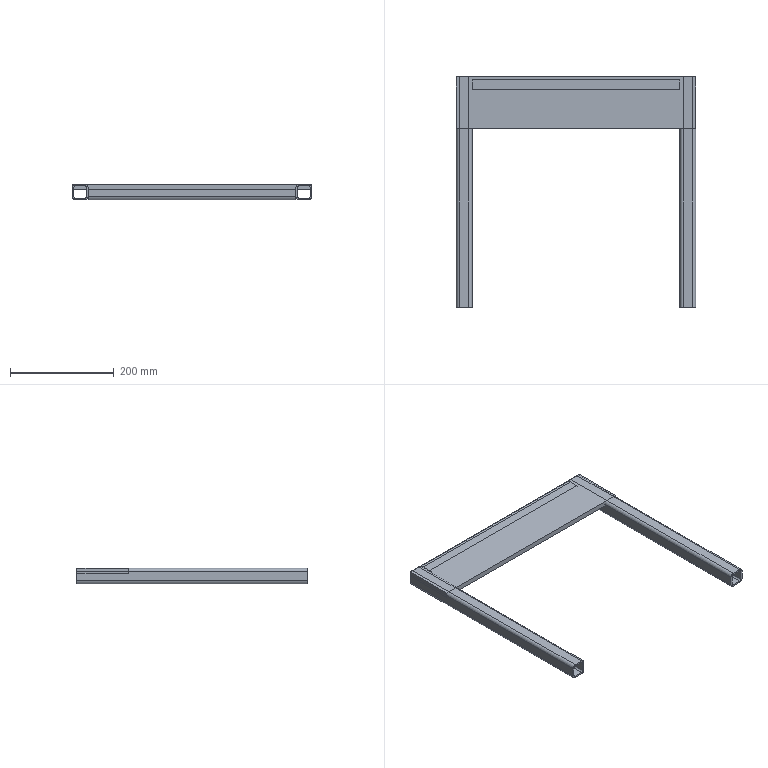Part | STEP file | MYT-A01-P40(Default_machined_) | 4 solids | 60 faces | box 460 x 443 x 30 mm | volume 846858 mm3 | plane 36 | cylinder 24 | commonest cylinder face diameters 6 x12 12 x12